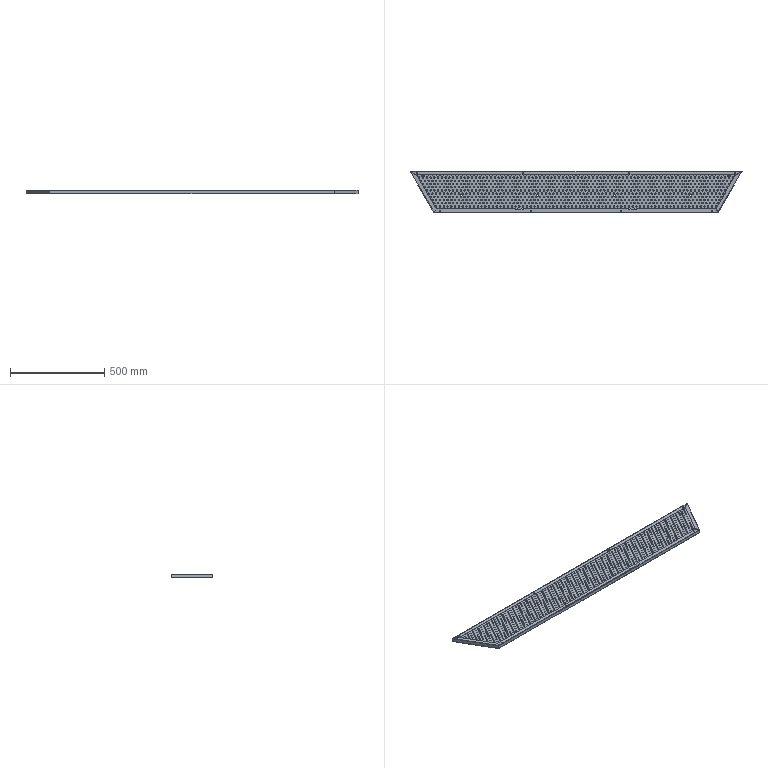Part | SolidWorks | features ICE 19, LPattern 12, EdgeFlange 4, FlatPattern 1, SMBaseFlange 1, SheetMetal 1 | 1 solid | 2057 faces | box 1758 x 220 x 20 mm | volume 678104 mm3 | cylinder 1958 | plane 88 | spline 11 | commonest cylinder face diameters 7.2 x1908 6 x18 6.4 x16 1 x8 4 x8